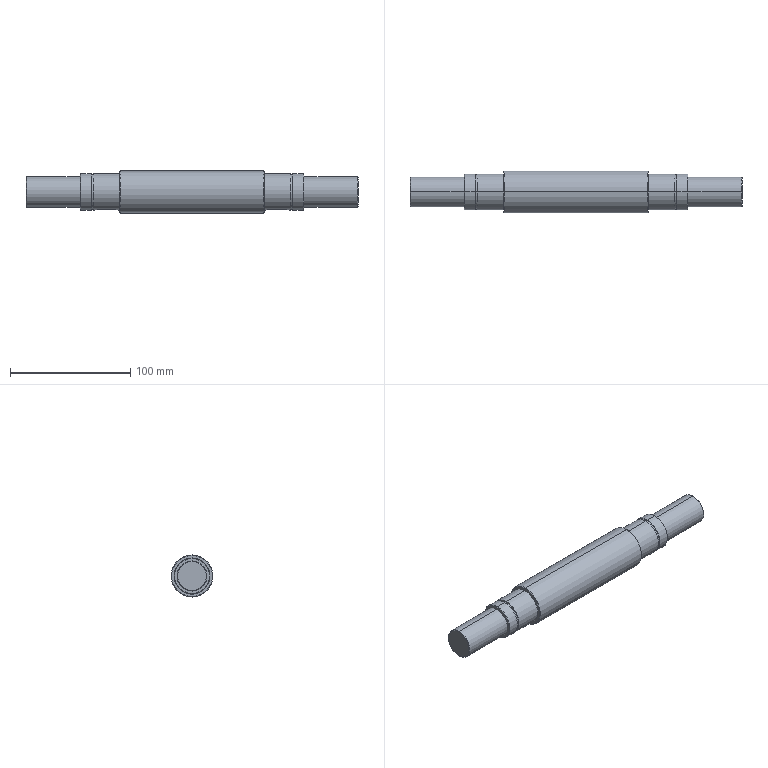Part | SolidWorks | features ICE 4, Chamfer 3, 3DProfileFeature 1, HoleWzd 1, MirrorPattern 1, Revolution 1 | 1 solid | 52 faces | box 276 x 35 x 35 mm | volume 204867 mm3 | cylinder 24 | plane 16 | cone 12 | commonest cylinder face diameters 30 x8 8 x6 25 x4 28.6 x4 35 x2